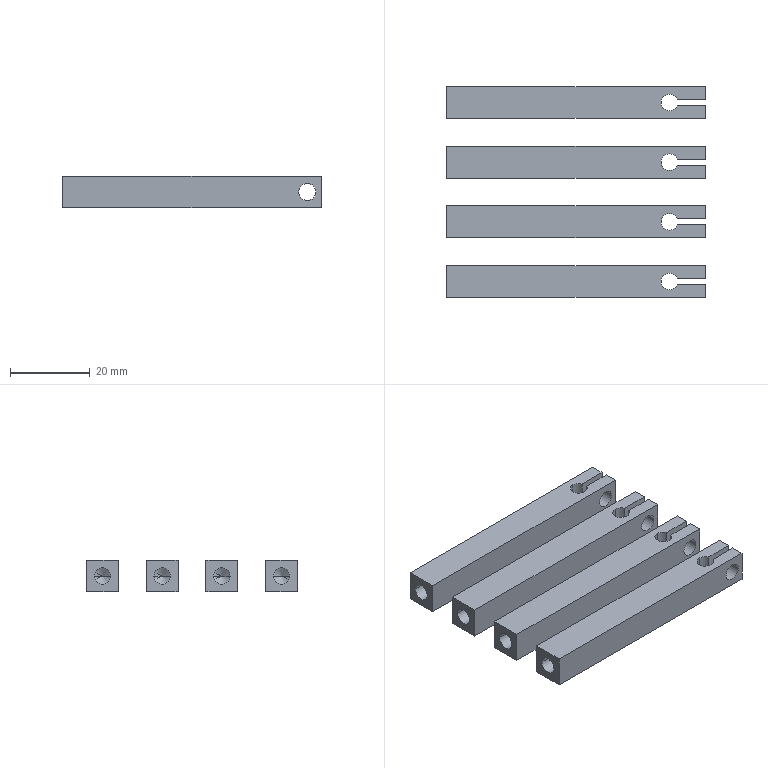NC program | NX | posted with a generic post | part box 65 x 53 x 8 mm
Whole program:
N10 G17 G21 G94 G90
(DRILLING_COPY , TOOL : D6A45)
N12 T07 M6
N14 G54
N16 G17 G0 G90 X29. Y0. B0. C0. S5000 M3
N18 G43 Z30. H7
N20 G94 G81 G98 Z-2.25 F250. R3.
N22 G80
N24 G0 X29. Y0. Z30.
N26 M5
(DRILLING_COPY_COPY_COPY , TOOL : 4.3ZT)
N28 T12 M6
N30 G54
N32 G17 G0 G90 X29. Y0. B0. C0. S2000 M3
N34 G43 Z30. H12
N36 G94 G83 G98 Z-9.792 F200. Q2. R3.
N38 G80
N40 G0 X29. Y0. Z30.
N42 M5
N44 M2